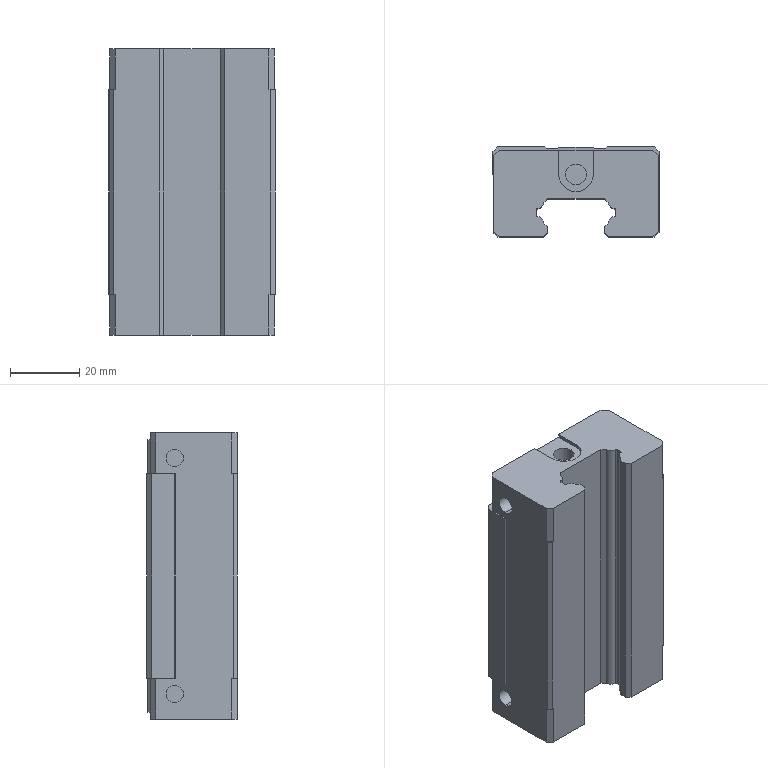Part | SolidWorks | features BaseBody 1 | 1 solid | 114 faces | box 48 x 26 x 82.6 mm | volume 80910 mm3 | plane 76 | cylinder 38 | commonest cylinder face diameters 6 x12 1 x8 5 x8 4 x4 7.3 x4 10 x2